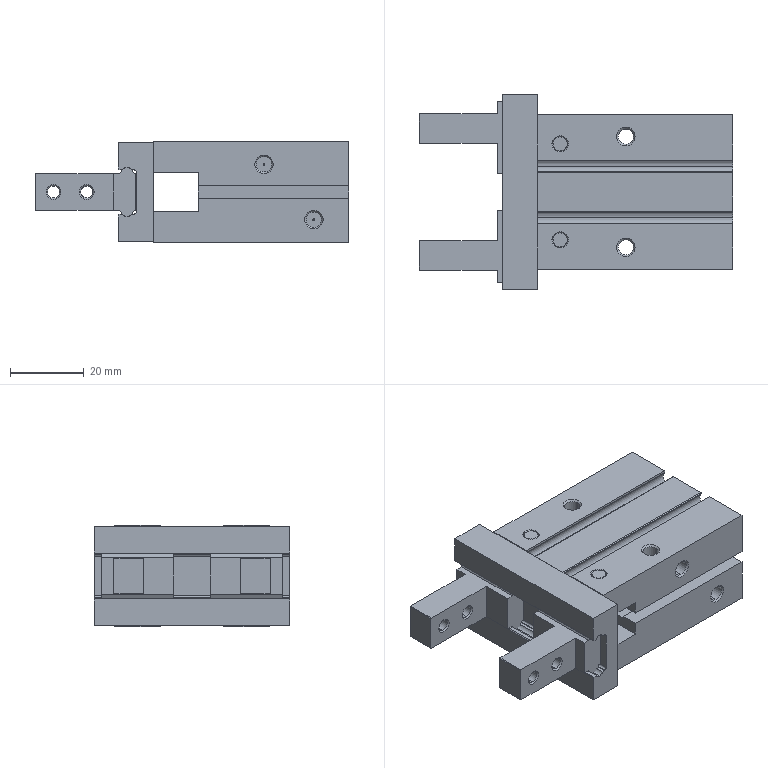Part | SolidWorks | 3 solids | 251 faces | box 85 x 53 x 27.5 mm | volume 63420 mm3 | plane 120 | cylinder 69 | cone 62 | commonest cylinder face diameters 4.134 x20 2.5 x9 0.4 x8 3.242 x8 5.02 x8 4.2 x6